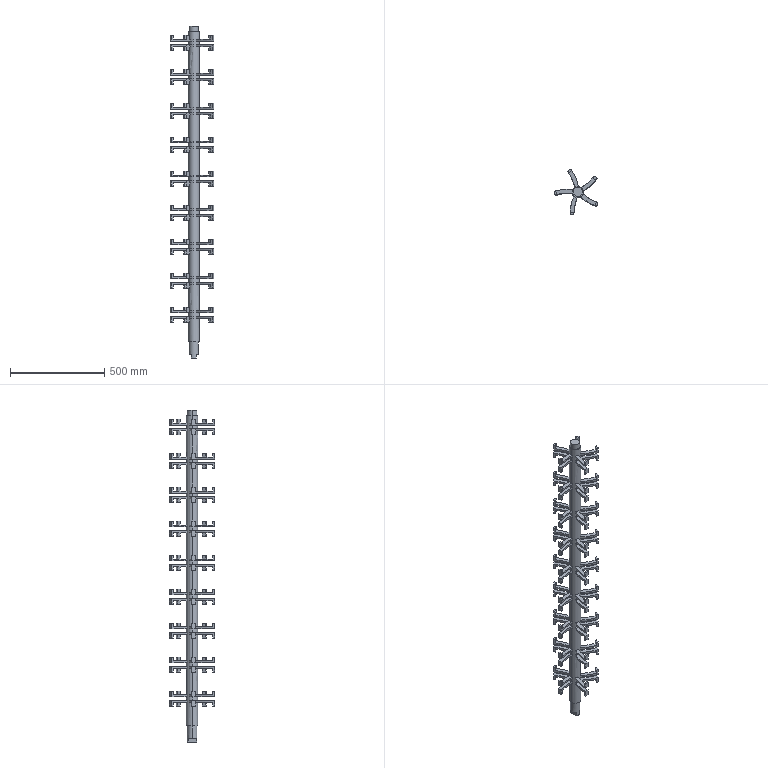Part | SolidWorks | 1 solid | 644 faces | box 232.128 x 238.99 x 1760 mm | volume 6921520 mm3 | plane 458 | cylinder 186 | commonest cylinder face diameters 508.027 x90 548.027 x90 50 x4 60 x2